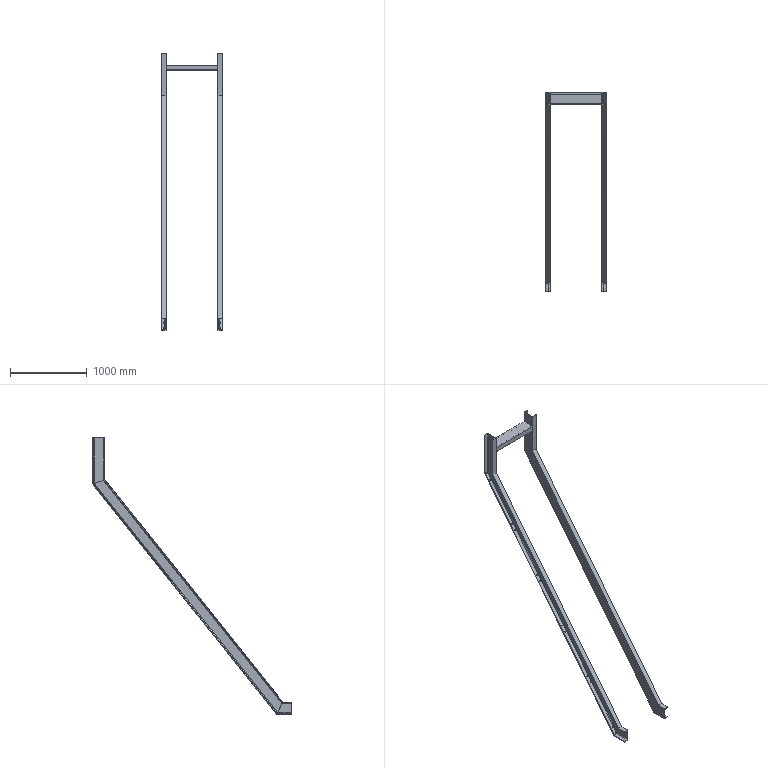Part | STEP file | Powder bin stair body_Default<As Machined> | 7 solids | 146 faces | box 800 x 2588 x 3603 mm | volume 21206724 mm3 | cylinder 76 | plane 70 | commonest cylinder face diameters 12 x48 10 x14 20 x14